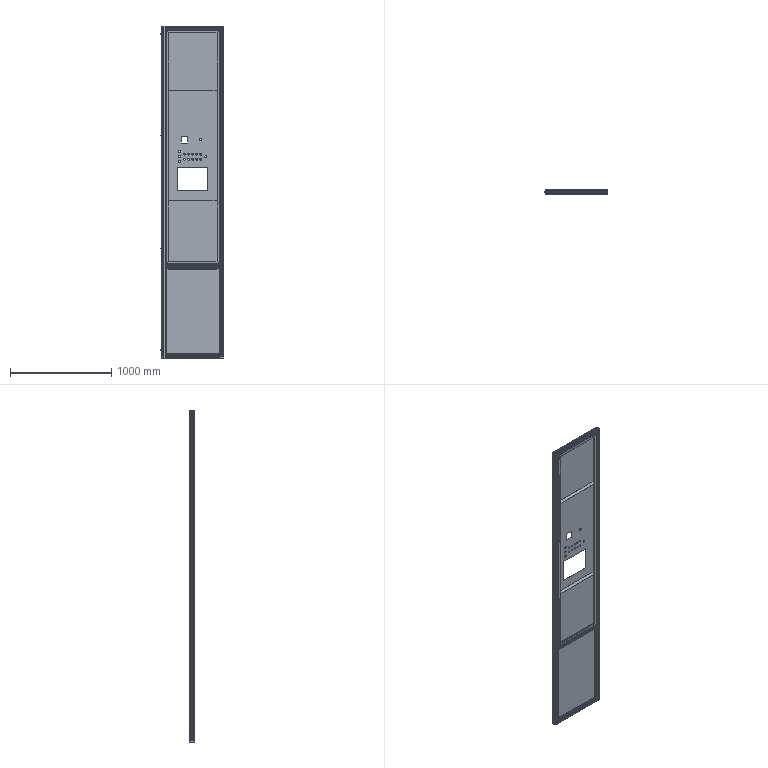Part | SolidWorks | 83 solids | 4063 faces | volume 9752547 mm3 | plane 2554 | cylinder 1141 | cone 272 | spline 96 | commonest cylinder face diameters 20.854 x128 0.562 x120 5 x104 6.8 x103 2 x58 1.6 x56